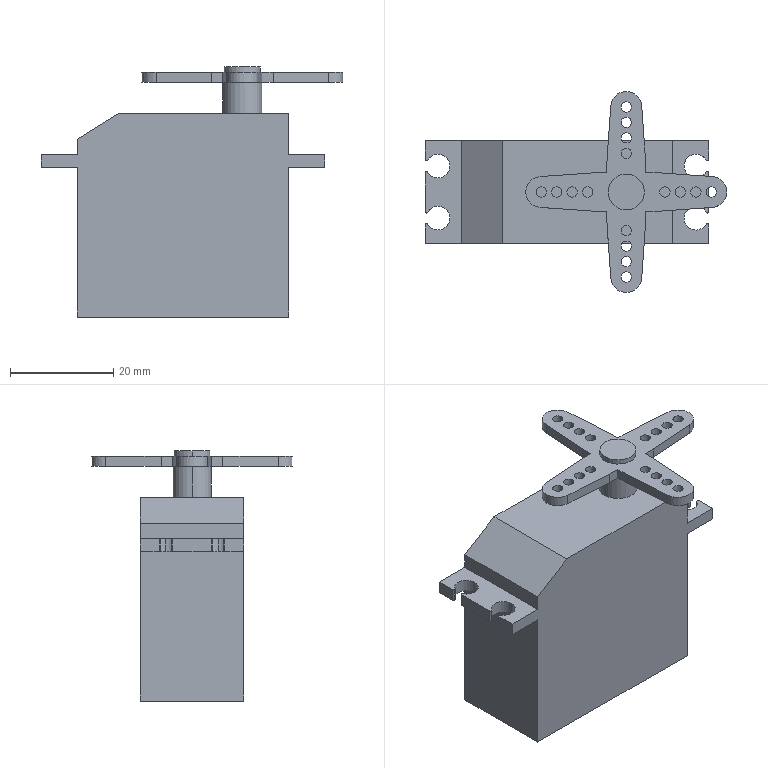Part | SolidWorks | features ICE 6, Fillet 2, Chamfer 1, Extrusion 1, MirrorPattern 1 | 1 solid | 100 faces | box 58.5 x 39 x 48.5 mm | volume 33649 mm3 | cylinder 61 | plane 39 | commonest cylinder face diameters 2 x32 0.6 x14 4.6 x6 6 x5 7 x2 7.5 x2